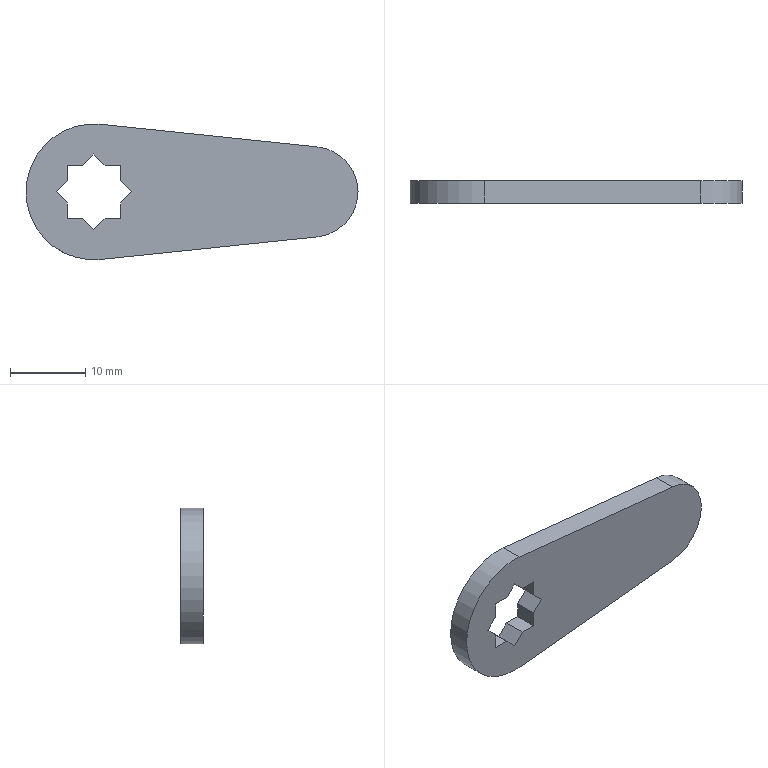Part | STEP file | _X2_751F4E45_X0_MS731-1_X2_8F_7 | 1 solid | 22 faces | box 44 x 3 x 18 mm | volume 1686 mm3 | plane 20 | cylinder 2 | commonest cylinder face diameters 12 x1 18 x1